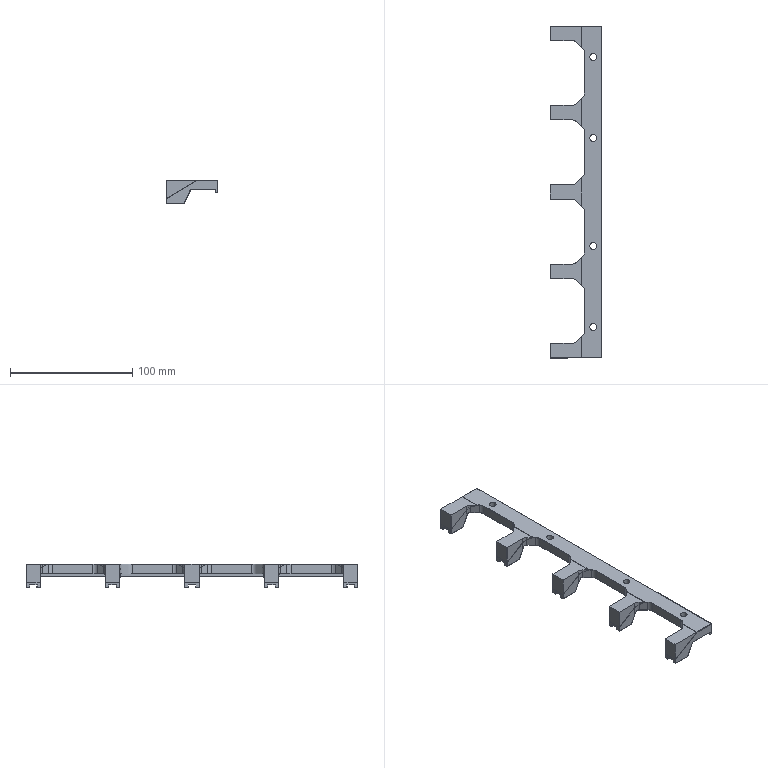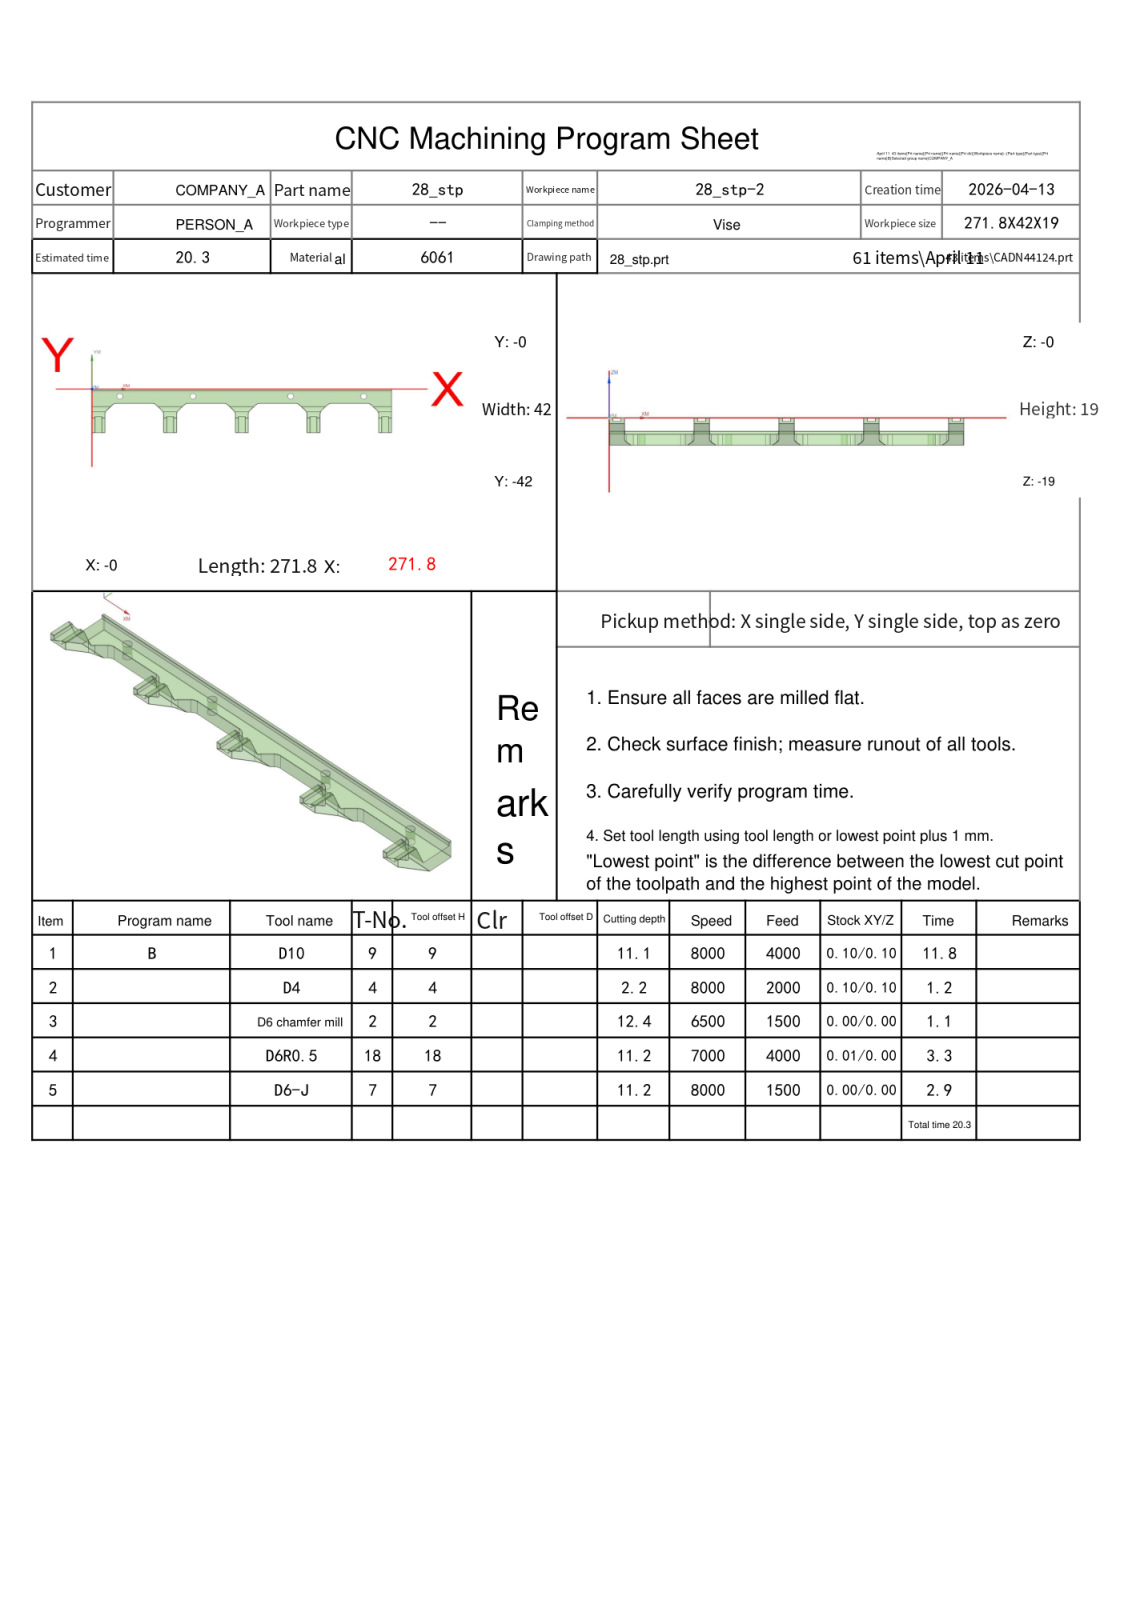NC program | NX | posted by the shop | part box 42 x 271.8 x 19 mm
Lines 1 to 789 of 14465:
%
O0001
(Machine time: 21.21 MIN)
(===Total Tool:5===)
(T9=D10     D=10.  R=0.   D-  H09 Z=-11.15)
(T4=D4      D=4.   R=0.   D-  H04 Z=-2.2  )
(T2=D6 chamfer mill   D=6.   R=0.   D-  H02 Z=-12.45)
(T18=D6R0.5 D=6.   R=0.5  D-  H18 Z=-11.25)
(T7=D6-J    D=6.   R=0.   D7  H07 Z=-11.25)
G80 G90 G17 G49 G40
G91 G28 Z0
M01
N1 T09 M06
(D10  D=10. R=0. H=09 ce=0.12 di=0.10)
G00 G90 G54 X-11.795 Y7.409 M03 S8000
G43 H09 Z20.
M08
Z2.1
G01 X-11.7 Y7.377 Z1.476 F4000.
X-11.606 Y7.345 Z1.228
X-11.511 Y7.313 Z1.046
X-11.416 Y7.281 Z.9
X-11.321 Y7.249 Z.777
X-11.227 Y7.218 Z.672
X-11.132 Y7.186 Z.58
X-11.037 Y7.154 Z.5
X-10.942 Y7.122 Z.43
X-10.847 Y7.09 Z.368
X-10.753 Y7.058 Z.314
X-10.658 Y7.026 Z.267
X-10.563 Y6.994 Z.227
X-10.468 Y6.962 Z.192
X-10.373 Y6.931 Z.164
X-10.279 Y6.899 Z.14
X-10.184 Y6.867 Z.123
X-10.089 Y6.835 Z.11
X-9.994 Y6.803 Z.103
X-9.9 Y6.771 Z.1
X-7.678 Y6.024
X-7.519 Y5.999
G03 X-7.265 Y6.065 I0.0 J.518
G02 X-4.273 Y7.054 I3.98 J-7.02
X1.978 Y7.487 I6.251 J-44.913
X2.707 Y7.481 I0.0 J-45.346
G01 X272.969 Y7.484
G02 X279.225 Y3.048 I-.106 J-6.778
X280.279 Y-2.628 I-16.186 J-5.943
X280.412 Y-11.519 I-296.3 J-8.891
X280.4 Y-14.276 I-296.434 J0.0
G01 X280.384 Y-42.069
G02 X275.948 Y-48.325 I-6.779 J.106
X270.272 Y-49.38 I-5.943 J16.179
X261.642 Y-49.511 I-8.63 J283.705
X259.174 Y-49.5 I0.0 J283.836
G01 X-1.169 Y-49.484
G02 X-7.425 Y-45.046 I.106 J6.779
X-8.479 Y-39.369 I16.195 J5.942
X-8.613 Y-30.479 I296.233 J8.891
X-8.6 Y-27.721 I296.367 J0.0
G01 X-8.579 Y.169
G02 X-5.27 Y5.129 I6.366 J-.663
X.261 Y6.734 I6.404 J-11.735
X8.124 Y7.016 I7.863 J-109.656
X10.104 Y6.998 I0.0 J-109.937
G01 X271.455 Y6.983
G02 X278.208 Y2.545 I-.199 J-7.66
X279.692 Y-3.639 I-15.009 J-6.873
X279.908 Y-11.563 I-145.435 J-7.924
X279.897 Y-13.335 I-145.651 J0.0
G01 X279.883 Y-40.554
G02 X275.445 Y-47.308 I-7.661 J.199
X269.26 Y-48.793 I-6.87 J14.988
X261.53 Y-49.006 I-7.73 J140.023
X259.965 Y-48.997 I0.0 J140.236
G01 X.346 Y-48.983
G02 X-6.409 Y-44.543 I.199 J7.66
X-7.892 Y-38.359 I14.999 J6.869
X-8.106 Y-30.635 I139.817 J7.723
X-8.097 Y-29.063 I140.03 J0.0
G01 X-8.074 Y-1.596
G02 X-3.705 Y4.686 I7.728 J-.715
X2.557 Y6.264 I7.074 J-14.863
X10.377 Y6.505 I7.82 J-126.46
X11.852 Y6.497 I0.0 J-126.702
G01 X270.151 Y6.476
G02 X277.677 Y1.337 I-.33 J-8.563
X279.179 Y-5.206 I-16.982 J-7.342
X279.406 Y-13.448 I-149.533 J-8.242
X279.396 Y-15.151 I-149.76 J0.0
G01 X279.375 Y-39.251
G02 X274.237 Y-46.777 I-8.564 J.33
X267.694 Y-48.279 I-7.34 J16.973
X259.451 Y-48.507 I-8.243 J149.431
X257.749 Y-48.497 I0.0 J149.659
G01 X1.649 Y-48.476
G02 X-5.878 Y-43.335 I.329 J8.563
X-7.379 Y-36.793 I16.987 J7.341
X-7.606 Y-28.55 I149.608 J8.243
X-7.597 Y-26.847 I149.835 J0.0
G01 X-7.583 Y-3.397
G02 X-2.472 Y4.191 I8.651 J-.311
X3.907 Y5.74 I7.394 J-16.544
X12.623 Y6.012 I8.716 J-139.521
X14.651 Y5.997 I0.0 J-139.793
G01 X268.651 Y5.98
G02 X277.155 Y.266 I-.078 J-9.301
X278.671 Y-6.584 I-18.644 J-7.719
X278.919 Y-16.462 I-196.83 J-9.878
X278.898 Y-19.329 I-197.078 J0.0
G01 X278.874 Y-37.879
G02 X273.167 Y-46.254 I-9.29 J.198
X266.317 Y-47.771 I-7.72 J18.631
X256.444 Y-48.02 I-9.873 J196.342
X253.572 Y-47.999 I0.0 J196.591
G01 X3.022 Y-47.974
G02 X-5.355 Y-42.265 I.197 J9.289
X-6.871 Y-35.416 I18.638 J7.719
X-7.119 Y-25.54 I196.76 J9.876
X-7.098 Y-22.67 I197.007 J0.0
G01 X-7.076 Y-4.721
G02 X-1.344 Y3.71 I9.379 J-.213
X5.45 Y5.252 I7.777 J-18.529
X14.088 Y5.506 I8.638 J-146.637
X15.795 Y5.496 I0.0 J-146.891
G01 X267.395 Y5.477
X267.455
G02 X276.622 Y-.684 I0.0 J-9.9
X278.154 Y-7.684 I-19.759 J-7.994
X278.414 Y-17.274 I-176.987 J-9.59
X278.397 Y-19.729 I-177.247 J0.0
X278.422 Y-26.265 I-849.199 J-6.536
X278.355 Y-36.928 I-849.224 J0.0
X272.171 Y-45.741 I-9.867 J.347
X265.217 Y-47.255 I-7.965 J19.865
X255.655 Y-47.514 I-9.562 J175.951
X253.222 Y-47.497 I0.0 J176.21
G01 X4.472 Y-47.48
X4.373
G02 X-4.901 Y-41.132 I0.0 J9.949
X-6.38 Y-33.967 I20.78 J8.025
X-6.61 Y-24.59 I191.061 J9.376
X-6.597 Y-22.321 I191.291 J0.0
X-6.623 Y-15.96 I780.546 J6.36
X-6.555 Y-5.645 I780.572 J0.0
X-.396 Y3.184 I9.936 J-.368
X6.8 Y4.757 I8.151 J-20.038
X16.203 Y5.011 I9.403 J-174.325
X18.395 Y4.997 I0.0 J-174.578
G01 X266.195 Y4.976
X266.308 Y4.977
G02 X273.054 Y2.608 I0.0 J-10.793
X276.86 Y-3.79 I-8.179 J-9.195
X277.795 Y-11.517 I-34.244 J-8.065
X277.918 Y-25.662 I-814.582 J-14.145
X277.856 Y-35.716 I-814.705 J0.0
X271.382 Y-45.169 I-10.365 J.155
X264.036 Y-46.753 I-8.341 J20.865
X254.233 Y-47.013 I-9.802 J184.172
X251.791 Y-46.997 I0.0 J184.433
G01 X5.691 Y-46.978
X5.535 Y-46.979
G02 X-.994 Y-44.818 I0.0 J10.942
X-5.025 Y-38.337 I7.733 J9.303
X-5.992 Y-30.565 I33.429 J8.107
X-6.119 Y-16.3 I800.504 J14.265
X-6.066 Y-7.066 I800.631 J0.0
X-2.953 Y.4 I10.54 J-.012
X3.803 Y3.699 I9.122 J-10.117
X12.12 Y4.443 I8.317 J-46.089
G01 X12.308
X23.358 Y4.498
X264.958 Y4.478
X265.132 Y4.479
G02 X271.26 Y2.813 I0.0 J-12.108
X276.047 Y-3.693 I-6.503 J-9.798
X277.251 Y-11.629 I-29.197 J-8.486
X277.41 Y-22.376 I-362.331 J-10.748
X277.398 Y-25.377 I-362.49 J0.0
X277.419 Y-28.555 I-231.25 J-3.178
X277.329 Y-35.025 I-231.271 J0.0
X270.515 Y-44.655 I-10.77 J.395
X263.264 Y-46.225 I-8.45 J21.495
X253.3 Y-46.513 I-9.964 J172.438
X250.92 Y-46.496 I0.0 J172.726
G01 X6.87 Y-46.478
X6.674 Y-46.48
G02 X.522 Y-44.801 I0.0 J12.114
X-4.265 Y-38.251 I6.536 J9.802
X-5.449 Y-30.413 I29.275 J8.428
X-5.612 Y-19.358 I374.413 J11.054
X-5.598 Y-16.114 I374.576 J0.0
X-5.62 Y-13.324 I170.908 J2.79
X-5.518 Y-7.416 I170.931 J0.0
X1.292 Y2.122 I10.815 J-.521
X8.787 Y3.734 I8.609 J-21.797
X18.671 Y4.011 I9.883 J-176.508
X20.932 Y3.996 I0.0 J-176.784
G01 X263.905 Y3.976
X264.088 Y3.977
G02 X270.164 Y2.482 I0.0 J-13.091
X275.365 Y-4.047 I-6.028 J-10.138
X276.713 Y-12.006 I-27.321 J-8.722
X276.917 Y-23.485 I-323.515 J-11.479
X276.897 Y-27.054 I-323.719 J0.0
X276.92 Y-29.233 I-104.221 J-2.18
X276.787 Y-34.501 I-104.244 J0.0
X269.875 Y-44.06 I-11.065 J.722
X262.191 Y-45.727 I-8.823 J22.133
X251.868 Y-46.013 I-10.323 J185.754
X249.347 Y-45.996 I0.0 J186.041
G01 X7.997 Y-45.978
G02 X7.765 Y-45.98 I-.231 J13.325
X1.768 Y-44.554 I0.0 J13.327
X-3.565 Y-37.952 I5.864 J10.192
X-4.893 Y-30.342 I26.599 J8.561
X-5.11 Y-19.961 I247.561 J10.381
X-5.097 Y-17.346 I247.779 J0.0
X-5.117 Y-14.552 I192.949 J2.793
X-5.022 Y-8.497 I192.97 J0.0
X-1.22 Y-.427 I11.218 J-.354
X5.74 Y2.7 I9.442 J-11.706
X14.298 Y3.434 I8.572 J-49.713
X23.691 Y3.501 I9.394 J-662.247
X25.697 Y3.498 I0.0 J-662.314
G01 X262.805 Y3.476
G02 X263.03 Y3.478 I.226 J-14.34
X269.016 Y2.17 I0.0 J-14.342
X274.731 Y-4.522 I-5.534 J-10.512
X276.159 Y-12.166 I-25.742 J-8.767
X276.408 Y-22.419 I-211.138 J-10.253
X276.395 Y-24.761 I-211.386 J0.0
X276.418 Y-27.455 I-156.525 J-2.694
X276.313 Y-33.209 I-156.548 J0.0
X273.046 Y-40.917 I-11.648 J.391
X266.214 Y-44.489 I-9.743 J10.319
X257.427 Y-45.412 I-8.907 J42.496
X246.757 Y-45.499 I-10.67 J655.992
X245.428 Y-45.497 I0.0 J656.079
G01 X8.978 Y-45.475
G02 X8.75 Y-45.477 I-.229 J14.212
X2.681 Y-44.117 I0.0 J14.213
X-2.918 Y-37.512 I5.642 J10.459
X-4.367 Y-29.724 I25.844 J8.838
X-4.609 Y-19.332 I222.743 J10.392
X-4.596 Y-16.878 I222.985 J0.0
X-4.618 Y-14.578 I117.791 J2.3
X-4.49 Y-9.081 I117.813 J0.0
X2.884 Y1.09 I11.518 J-.592
X10.332 Y2.695 I8.839 J-22.927
X20.903 Y3.014 I10.571 J-175.375
X23.425 Y2.995 I0.0 J-175.694
G01 X261.905 Y2.973
G02 X262.115 Y2.974 I.21 J-15.017
X268.267 Y1.656 I0.0 J-15.019
X274.158 Y-5.138 I-5.544 J-10.758
X275.637 Y-12.82 I-25.698 J-8.931
X275.906 Y-23.079 I-195.35 J-10.259
X275.894 Y-25.265 I-195.619 J0.0
X275.919 Y-27.43 I-95.331 J-2.165
X275.767 Y-32.811 I-95.356 J0.0
X268.294 Y-43.045 I-11.723 J.715
X260.353 Y-44.717 I-9.163 J23.825
X249.624 Y-45.012 I-10.729 J194.642
X247.059 Y-44.995 I0.0 J194.938
G01 X10.009 Y-44.975
G02 X9.755 Y-44.978 I-.255 J15.393
X3.726 Y-43.748 I0.0 J15.396
X-2.268 Y-37.094 I5.258 J10.763
X-3.837 Y-29.179 I25.069 J9.084
X-4.108 Y-18.729 I201.282 J10.45
X-4.095 Y-16.385 I201.553 J0.0
X-4.12 Y-14.517 I67.551 J1.868
X-3.922 Y-9.341 I67.577 J0.0
X3.602 Y.559 I11.731 J-1.107
X11.546 Y2.217 I9.178 J-24.114
X21.562 Y2.504 I10.015 J-174.607
X23.441 Y2.494 I0.0 J-174.894
G01 X260.755 Y2.477
G02 X261.039 Y2.479 I.285 J-16.818
X266.973 Y1.398 I0.0 J-16.821
X273.468 Y-5.437 I-4.84 J-11.103
X275.122 Y-13.538 I-25.006 J-9.323
X275.41 Y-24.378 I-203.341 J-10.84
X275.394 Y-26.932 I-203.629 J0.0
X275.417 Y-28.254 I-38.553 J-1.322
X275.084 Y-33.316 I-38.576 J0.0
X267.811 Y-42.421 I-11.724 J1.908
X260.138 Y-44.157 I-9.207 J22.861
X249.958 Y-44.503 I-10.18 J149.811
X248.097 Y-44.491 I0.0 J150.157
G01 X10.847 Y-44.471
G02 X10.626 Y-44.473 I-.221 J15.999
X4.462 Y-43.238 I0.0 J16.
X-1.762 Y-36.33 I5.305 J11.037
X-3.325 Y-28.411 I25.671 J9.182
X-3.61 Y-17.523 I207.847 J10.888
X-3.518 Y-11.318 I208.132 J0.0
X-1.305 Y-4.308 I13.227 J-.322
X5.76 Y.56 I10.658 J-7.907
X14.093 Y1.82 I9.163 J-32.428
X24.897 Y2.006 I10.804 J-312.688
X27.39 Y1.996 I0.0 J-312.874
G01 X259.655 Y1.979
G02 X260.007 Y1.983 I.352 J-18.624
X265.853 Y1.041 I0.0 J-18.627
X272.898 Y-6.019 I-4.401 J-11.437
X274.593 Y-14.06 I-24.769 J-9.42
X274.906 Y-24.501 I-173.985 J-10.441
X274.797 Y-30.652 I-174.298 J0.0
X272.374 Y-37.853 I-13.237 J.446
X265.423 Y-42.529 I-10.66 J8.341
X256.843 Y-43.821 I-9.368 J33.069
X244.891 Y-44.013 I-11.951 J372.933
X241.395 Y-43.996 I0.0 J373.125
G01 X11.845 Y-43.972
G02 X11.581 Y-43.974 I-.264 J17.171
X5.389 Y-42.819 I0.0 J17.173
X-1.193 Y-35.748 I5.067 J11.315
X-2.793 Y-27.939 I25.367 J9.266
X-3.099 Y-17.692 I171.118 J10.247
X-3.006 Y-12.047 I171.425 J0.0
X-.751 Y-4.932 I13.547 J-.379
X6.244 Y-.032 I10.784 J-7.953
X14.415 Y1.287 I9.237 J-31.246
X25.947 Y1.513 I11.532 J-294.663
X29.112 Y1.496 I0.0 J-294.889
G01 X258.862 Y1.476
G02 X259.212 Y1.479 I.351 J-18.864
X265.347 Y.454 I0.0 J-18.867
X272.345 Y-6.626 I-4.624 J-11.569
X274.075 Y-14.709 I-24.857 J-9.547
X274.394 Y-24.373 I-146.526 J-9.663
X274.292 Y-29.85 I-146.844 J0.0
X271.94 Y-37.079 I-13.678 J.453
X264.819 Y-41.98 I-10.907 J8.221
X256.295 Y-43.303 I-9.448 J32.751
X244.601 Y-43.511 I-11.694 J328.735
X241.398 Y-43.496 I0.0 J328.943
G01 X13.148 Y-43.48
G02 X12.741 Y-43.484 I-.407 J20.026
X6.838 Y-42.594 I0.0 J20.03
X-.545 Y-35.373 I4.21 J11.69
X-2.275 Y-27.29 I24.856 J9.546
X-2.59 Y-17.957 I138.294 J9.332
X-2.49 Y-12.699 I138.609 J0.0
X-.148 Y-5.47 I13.742 J-.46
X6.955 Y-.545 I10.936 J-8.186
X15.577 Y.803 I9.529 J-32.693
X27.763 Y1.015 I12.186 J-351.327
X31.374 Y.996 I0.0 J-351.538
G01 X258.124 Y.972
G02 X258.427 Y.975 I.303 J-19.32
X264.66 Y-.058 I0.0 J-19.323
X271.866 Y-7.394 I-4.675 J-11.8
X273.579 Y-15.589 I-25.787 J-9.668
X273.887 Y-23.974 I-114.061 J-8.386
X273.757 Y-29.429 I-114.368 J0.0
X271.04 Y-36.938 I-13.49 J.634
X263.709 Y-41.594 I-10.961 J9.159
X255.116 Y-42.819 I-9.484 J35.776
X243.422 Y-43.009 I-11.693 J360.837
X240.318 Y-42.995 I0.0 J361.026
G01 X13.818 Y-42.975
G02 X13.484 Y-42.978 I-.334 J20.139
X7.414 Y-42.042 I0.0 J20.142
X.011 Y-34.79 I4.341 J11.837
X-1.736 Y-26.908 I24.518 J9.568
X-2.077 Y-18.213 I110.618 J8.696
X-1.967 Y-13.269 I110.96 J0.0
X.6 Y-5.803 I13.757 J-.556
X7.78 Y-1.016 I11.006 J-8.728
X16.608 Y.312 I9.687 J-34.392
X28.879 Y.513 I12.271 J-374.296
X32.506 Y.496 I0.0 J-374.497
G01 X257.105 Y.475
G02 X257.479 Y.478 I.374 J-20.932
X263.709 Y-.47 I0.0 J-20.935
X271.264 Y-7.851 I-4.361 J-12.02
X273.025 Y-15.777 I-24.796 J-9.67
X273.368 Y-23.848 I-94.987 J-8.071
X273.241 Y-28.765 I-95.329 J0.0
X270.383 Y-36.48 I-13.646 J.668
X263.117 Y-41.054 I-11.013 J9.437
X254.429 Y-42.312 I-9.626 J35.863
X242.438 Y-42.51 I-11.991 J361.696
X239.131 Y-42.495 I0.0 J361.895
G01 X14.582 Y-42.472
G02 X14.25 Y-42.475 I-.331 J20.452
X7.984 Y-41.492 I0.0 J20.455
X.536 Y-34.148 I4.474 J11.987
X-1.225 Y-26.221 I24.804 J9.67
X-1.56 Y-18.463 I89.769 J7.758
X-1.438 Y-13.783 I90.104 J0.0
X1.31 Y-6.185 I13.752 J-.679
X8.625 Y-1.478 I11.102 J-9.213
X17.26 Y-.197 I9.636 J-35.228
X29.588 Y.013 I12.328 J-361.145
X33.157 Y-.005 I0.0 J-361.355
G01 X256.257 Y-.025
G02 X256.641 Y-.022 I.384 J-21.962
X262.918 Y-.938 I0.0 J-21.965
X270.752 Y-8.512 I-4.26 J-12.246
X272.545 Y-16.786 I-25.686 J-9.896
X272.843 Y-23.698 I-79.8 J-6.912
X272.721 Y-28.125 I-80.098 J0.0
X269.844 Y-35.884 I-13.824 J.714
X262.41 Y-40.552 I-11.184 J9.555
X253.519 Y-41.816 I-9.785 J36.946
X240.923 Y-42.012 I-12.597 J403.156
X237.172 Y-41.995 I0.0 J403.353
G01 X15.572 Y-41.975
G02 X15.178 Y-41.978 I-.394 J22.095
X8.91 Y-41.071 I0.0 J22.099
X1.048 Y-33.487 I4.231 J12.254
X-.722 Y-25.462 I25.29 J9.787
X-1.038 Y-18.742 I71.335 J6.719
X-.889 Y-14.125 I71.651 J0.0
X2.437 Y-6.088 I13.46 J-.864
X9.987 Y-1.793 I11.065 J-10.666
X19.15 Y-.649 I9.828 J-41.452
X30.542 Y-.499 I11.392 J-434.014
X32.848 Y-.505 I0.0 J-434.163
G01 X255.098 Y-.52
G02 X255.595 Y-.515 I.497 J-24.834
X261.781 Y-1.298 I0.0 J-24.839
X270.19 Y-9.041 I-3.761 J-12.521
X272.031 Y-17.405 I-25.68 J-10.038
X272.318 Y-23.433 I-63.226 J-6.028
X272.164 Y-27.843 I-63.513 J0.0
X268.641 Y-36.051 I-13.485 J.929
X261.267 Y-40.176 I-11.01 J11.026
X252.109 Y-41.343 I-9.893 J41.149
X239.832 Y-41.506 I-12.277 J460.42
X236.561 Y-41.495 I0.0 J460.583
G01 X16.211 Y-41.471
G02 X15.887 Y-41.473 I-.324 J22.324
X9.551 Y-40.555 I0.0 J22.327
X1.61 Y-32.958 I4.246 J12.386
X-.231 Y-24.594 I25.683 J10.038
X-.509 Y-18.952 I57.129 J5.641
X-.333 Y-14.458 I57.407 J0.0
X3.94 Y-5.721 I13.217 J-1.051
X11.597 Y-2.072 I10.862 J-12.934
X20.784 Y-1.119 I9.751 J-49.243
X32.79 Y-1.001 I12.006 J-611.267
X35.033 Y-1.005 I0.0 J-611.385
G01 X254.833 Y-1.031
G02 X255.161 Y-1.028 I.328 J-22.802
X261.642 Y-1.968 I0.0 J-22.804
X269.612 Y-9.526 I-4.277 J-12.493
X271.5 Y-17.828 I-25.254 J-10.11
X271.784 Y-23.209 I-50.985 J-5.38
X271.598 Y-27.563 I-51.268 J0.0
X266.537 Y-36.874 I-13.169 J1.127
X258.835 Y-40.076 I-10.698 J14.867
X248.833 Y-40.919 I-10.085 J59.858
X238.679 Y-40.996 I-10.153 J670.923
X236.933 Y-40.994 I0.0 J671.
G01 X17.083 Y-40.971
G02 X16.705 Y-40.974 I-.378 J23.254
X10.221 Y-40.052 I0.0 J23.257
X2.188 Y-32.473 I4.216 J12.516
X.304 Y-24.221 I25.172 J10.087
X.029 Y-19.158 I46.457 J5.063
X.239 Y-14.737 I46.732 J0.0
X8.483 Y-3.781 I13.175 J-1.333
X16.84 Y-1.893 I10.143 J-25.469
X27.614 Y-1.506 I10.775 J-149.721
X29.13 Y-1.514 I0.0 J-150.108
G01 X253.98 Y-1.53
G02 X254.344 Y-1.527 I.364 J-23.886
X260.894 Y-2.442 I0.0 J-23.889
X269.12 Y-10.201 I-4.194 J-12.686
X270.981 Y-18.365 I-25.435 J-10.092
X271.24 Y-23.021 I-41.625 J-4.656
X271.021 Y-27.298 I-41.884 J0.0
X262.748 Y-38.196 I-13.235 J1.458
X254.394 Y-40.095 I-10.196 J25.53
X243.374 Y-40.495 I-11.02 J151.412
X241.654 Y-40.485 I0.0 J151.812
G01 X18.204 Y-40.477
G02 X17.719 Y-40.481 I-.485 J26.141
X11.369 Y-39.698 I0.0 J26.145
X2.68 Y-31.798 I3.722 J12.821
X.789 Y-23.292 I25.918 J10.227
X.574 Y-19.32 I36.568 J3.972
X.851 Y-14.811 I36.784 J0.0
X9.025 Y-4.33 I13.164 J-1.839
X17.175 Y-2.432 I10.131 J-25.049
X28.289 Y-2.005 I11.114 J-144.273
X29.964 Y-2.014 I0.0 J-144.701
G01 X253.214 Y-2.03
G02 X253.584 Y-2.027 I.371 J-24.668
X260.181 Y-2.926 I0.0 J-24.671
X268.556 Y-10.702 I-4.109 J-12.823
X270.496 Y-19.298 I-25.697 J-10.316
X270.692 Y-22.857 I-32.272 J-3.559
X270.369 Y-27.425 I-32.468 J0.0
X262.164 Y-37.667 I-13.183 J2.154
X253.56 Y-39.604 I-10.372 J25.987
X242.602 Y-39.992 I-10.958 J154.469
X241.019 Y-39.984 I0.0 J154.857
G01 X18.619 Y-39.97
G02 X18.241 Y-39.973 I-.379 J24.856
X11.65 Y-39.083 I0.0 J24.859
X3.244 Y-31.297 I4.078 J12.833
X1.316 Y-22.801 I25.463 J10.246
X1.13 Y-19.477 I29.725 J3.324
X1.494 Y-14.827 I29.911 J0.0
X9.431 Y-4.938 I13.09 J-2.376
X17.862 Y-2.936 I10.358 J-24.863
X29.274 Y-2.501 I11.412 J-149.662
X31.201 Y-2.514 I0.0 J-150.097
G01 X252.451 Y-2.531
G02 X252.796 Y-2.528 I.345 J-25.909
X259.329 Y-3.366 I0.0 J-25.912
X268.079 Y-11.395 I-3.91 J-13.043
X270.022 Y-20.499 I-26.463 J-10.407
X270.135 Y-22.829 I-23.977 J-2.33
X269.551 Y-28.102 I-24.09 J0.0
X261.705 Y-37.085 I-12.939 J3.383
X253.468 Y-39.044 I-10.297 J25.003
X241.998 Y-39.496 I-11.47 J145.119
X240.13 Y-39.484 I0.0 J145.571
G01 X19.431 Y-39.47
G02 X19.055 Y-39.473 I-.375 J26.33
X12.549 Y-38.657 I0.0 J26.333
X3.721 Y-30.604 I3.832 J13.066
X1.788 Y-21.499 I26.123 J10.305
X1.691 Y-19.449 I21.654 J2.05
X2.433 Y-13.817 I21.751 J0.0
X10.162 Y-5.398 I12.802 J-3.996
X18.652 Y-3.428 I10.408 J-25.577
X29.787 Y-3.008 I11.134 J-147.205
X31.392 Y-3.016 I0.0 J-147.625
G01 X251.341 Y-3.025
G02 X251.84 Y-3.021 I.498 J-28.443
X258.43 Y-3.794 I0.0 J-28.447
X267.508 Y-11.864 I-3.62 J-13.213
X269.497 Y-21.359 I-25.617 J-10.323
X269.557 Y-22.861 I-18.894 J-1.502
X268.537 Y-28.994 I-18.954 J0.0
X261.024 Y-36.604 I-12.606 J4.932
X252.426 Y-38.577 I-10.488 J25.989
X240.877 Y-38.997 I-11.549 J158.47
X238.937 Y-38.985 I0.0 J158.89
G01 X20.387 Y-38.973
G02 X19.909 Y-38.977 I-.477 J27.972
X13.301 Y-38.186 I0.0 J27.976
X4.292 Y-30.135 I3.688 J13.193
X2.309 Y-19.948 I25.176 J10.187
X2.583 Y-16.102 I27.159 J0.0
X10.569 Y-6.001 I13.201 J-2.229
X18.991 Y-3.965 I10.474 J-24.883
X29.836 Y-3.518 I10.845 J-131.274
X30.979 Y-3.523 I0.0 J-131.722
G01 X250.778 Y-3.528
G02 X251.222 Y-3.525 I.444 J-28.201
X257.914 Y-4.33 I0.0 J-28.204
X267.054 Y-12.599 I-3.754 J-13.337
X268.926 Y-22.241 I-23.907 J-9.643
X268.679 Y-25.799 I-25.778 J0.0
X260.839 Y-35.901 I-13.194 J2.146
X252.284 Y-38.021 I-10.608 J24.486
X241.176 Y-38.485 I-11.109 J132.924
X239.848 Y-38.478 I0.0 J133.387
G01 X21.148 Y-38.473
G02 X20.66 Y-38.477 I-.488 J28.958
X14.008 Y-37.703 I0.0 J28.962
X4.746 Y-29.4 I3.631 J13.368
X2.918 Y-20.116 I22.658 J9.284
X3.186 Y-16.498 I24.486 J0.0
X11.116 Y-6.541 I13.168 J-2.35
X19.585 Y-4.475 I10.551 J-24.866
X30.654 Y-4.016 I11.069 J-133.105
X31.922 Y-4.022 I0.0 J-133.564
G01 X249.821 Y-4.025
G02 X250.341 Y-4.021 I.519 J-30.5
X257.016 Y-4.76 I0.0 J-30.504
X266.545 Y-13.199 I-3.475 J-13.523
X268.308 Y-22.071 I-21.436 J-8.872
X268.06 Y-25.456 I-23.2 J0.0
X260.338 Y-35.341 I-13.13 J2.299
X251.842 Y-37.495 I-10.645 J24.155
X240.846 Y-37.978 I-10.997 J124.902
X239.757 Y-37.974 I0.0 J125.385
G01 X21.907 Y-37.973
G02 X21.418 Y-37.977 I-.489 J30.166
X14.763 Y-37.234 I0.0 J30.17
X5.255 Y-28.798 I3.493 J13.512
X3.544 Y-20.263 I20.43 J8.535
X3.796 Y-16.935 I22.142 J0.0
X11.53 Y-7.14 I13.088 J-2.384
X20.074 Y-4.996 I10.665 J-24.398
X31.321 Y-4.515 I11.246 J-131.404
X32.66 Y-4.522 I0.0 J-131.884
G01 X249.16 Y-4.526
G02 X249.651 Y-4.522 I.491 J-31.109
X256.357 Y-5.253 I0.0 J-31.113
X266.045 Y-13.82 I-3.428 J-13.639
X267.673 Y-21.885 I-19.168 J-8.065
X267.392 Y-25.29 I-20.795 J0.0
X259.923 Y-34.74 I-12.981 J2.584
X251.498 Y-36.958 I-10.697 J23.52
X239.969 Y-37.484 I-11.529 J125.997
X238.514 Y-37.476 I0.0 J126.524
G01 X22.315 Y-37.467
G02 X21.908 Y-37.47 I-.407 J28.784
X15.081 Y-36.649 I0.0 J28.787
X5.814 Y-28.315 I3.761 J13.502
X4.188 Y-20.457 I18.179 J7.858
X4.492 Y-17.001 I19.804 J0.0
X11.937 Y-7.745 I12.913 J-2.765
X20.366 Y-5.539 I10.693 J-23.644
X31.406 Y-5.025 I11.04 J-118.368
X32.35 Y-5.029 I0.0 J-118.881
G01 X248.6
G02 X249.084 Y-5.025 I.484 J-30.351
X255.988 Y-5.821 I0.0 J-30.355
X265.506 Y-14.349 I-3.638 J-13.635
X267.017 Y-21.707 I-17.155 J-7.359
X266.692 Y-25.176 I-18.667 J0.0
X259.434 Y-34.173 I-12.814 J2.912
X250.923 Y-36.447 I-10.783 J23.295
X239.517 Y-36.98 I-11.406 J121.821
X238.24 Y-36.973 I0.0 J122.354
G01 X23.29 Y-36.972
G02 X22.81 Y-36.975 I-.48 J31.474
X16.044 Y-36.239 I0.0 J31.477
X6.275 Y-27.594 I3.41 J13.695
X4.853 Y-20.624 I16.368 J6.969
X5.194 Y-17.157 I17.79 J0.0
X12.441 Y-8.306 I12.735 J-3.034
X20.864 Y-6.059 I10.738 J-23.341
X32.137 Y-5.523 I11.274 J-118.426
X33.196 Y-5.528 I0.0 J-118.961
G01 X248.096 Y-5.533
G02 X248.482 Y-5.53 I.386 J-30.421
X255.337 Y-6.312 I0.0 J-30.424
X265.078 Y-15.164 I-3.591 J-13.739
X266.342 Y-21.534 I-15.43 J-6.371
X265.941 Y-25.169 I-16.694 J0.0
X258.788 Y-33.683 I-12.632 J3.351
X250.275 Y-35.945 I-10.794 J23.473
X239.181 Y-36.471 I-11.095 J116.747
X238.292 Y-36.467 I0.0 J117.273
G01 X23.843 Y-36.469
G02 X23.379 Y-36.472 I-.463 J30.819
X16.453 Y-35.684 I0.0 J30.822
X6.643 Y-26.607 I3.611 J13.742
X5.538 Y-20.806 I14.675 J5.801
X6.021 Y-16.932 I15.779 J0.0
X12.878 Y-8.901 I12.447 J-3.686
X21.281 Y-6.588 I10.786 J-22.761
X32.618 Y-6.026 I11.337 J-113.97
X33.662 Y-6.031 I0.0 J-114.533
G01 X247.162 Y-6.029
G02 X247.647 Y-6.025 I.485 J-32.43
X254.558 Y-6.77 I0.0 J-32.434
X264.653 Y-16.029 I-3.383 J-13.821
X265.645 Y-21.354 I-13.79 J-5.324
X265.008 Y-25.646 I-14.783 J0.0
X258.124 Y-33.2 I-12.323 J4.316
X249.798 Y-35.423 I-10.719 J23.442
X238.263 Y-35.977 I-11.535 J119.726
X237.017 Y-35.971 I0.0 J120.281
G01 X24.467 Y-35.967
G02 X24.008 Y-35.971 I-.458 J30.903
X16.98 Y-35.161 I0.0 J30.906
X6.964 Y-25.368 I3.661 J13.762
X6.24 Y-20.976 I12.953 J4.391
X7.322 Y-15.643 I13.677 J0.0
X14.285 Y-9.031 I12.097 J-5.768
X22.61 Y-7.012 I10.587 J-25.467
X33.638 Y-6.528 I11.028 J-125.404
X34.445 Y-6.53 I0.0 J-125.888
G01 X246.245 Y-6.526
G02 X246.832 Y-6.521 I.587 J-34.322
X253.845 Y-7.245 I0.0 J-34.327
X264.52 Y-18.053 I-3.258 J-13.895
X264.938 Y-21.259 I-12.076 J-3.206
X262.359 Y-28.863 I-12.494 J0.0
X254.956 Y-33.718 I-11.66 J9.706
X245.752 Y-35.222 I-10.623 J36.111
X233.439 Y-35.5 I-12.313 J272.108
X230.907 Y-35.488 I0.0 J272.387
G01 X25.457 Y-35.471
G02 X24.912 Y-35.476 I-.544 J33.892
X17.957 Y-34.755 I0.0 J33.896
X7.014 Y-21.012 I3.156 J13.742
X7.252 Y-18.433 I14.1 J0.0
X13.6 Y-10.194 I12.103 J-2.76
X21.885 Y-7.681 I10.858 J-20.886
X32.939 Y-7.046 I11.054 J-95.893
X33.411 Y-7.047 I0.0 J-96.528
G01 X44.911 Y-7.009
X245.56 Y-7.027
G02 X246.123 Y-7.022 I.562 J-35.676
X253.065 Y-7.704 I0.0 J-35.68
X264.136 Y-21.277 I-2.786 J-13.573
X264.055 Y-22.772 I-13.856 J0.0
X257.998 Y-31.577 I-11.98 J1.755
X249.766 Y-34.251 I-10.931 J19.641
X238.824 Y-34.941 I-10.942 J86.522
G01 X238.595 Y-34.94
X227.145 Y-34.99
X26.145 Y-34.971
G02 X25.567 Y-34.976 I-.578 J34.215
X18.497 Y-34.238 I0.0 J34.22
X7.775 Y-20.905 I2.929 J13.333
X7.778 Y-20.644 I13.651 J0.0
X13.455 Y-11.169 I11.778 J-.618
X21.428 Y-8.351 I10.892 J-18.131
X32.406 Y-7.571 I10.978 J-76.87
G01 X32.49
X43.74 Y-7.51
X244.84 Y-7.526
G02 X245.45 Y-7.521 I.61 J-36.246
X252.494 Y-8.212 I0.0 J-36.252
X263.16 Y-18.878 I-2.729 J-13.394
X263.352 Y-20.965 I-11.249 J-2.087
X258.246 Y-30.492 I-11.441 J0.0
X250.51 Y-33.514 I-10.91 J16.513
X239.759 Y-34.406 I-10.917 J66.377
X228.198 Y-34.496 I-11.561 J738.129
X225.16 Y-34.49 I0.0 J738.22
G01 X26.86 Y-34.471
G02 X26.301 Y-34.476 I-.558 J35.853
X19.306 Y-33.787 I0.0 J35.857
X9.288 Y-25.257 I2.713 J13.334
X8.593 Y-21.369 I10.53 J3.888
X13.472 Y-12.11 I11.225 J0.0
X21.274 Y-8.997 I10.939 J-16.079
X31.975 Y-8.096 I10.905 J-65.52
X43.363 Y-8.005 I11.388 J-715.518
X45.924 Y-8.01 I0.0 J-715.608
G01 X244.474 Y-8.031
G02 X244.955 Y-8.028 I.481 J-35.356
X251.977 Y-8.732 I0.0 J-35.359
X261.384 Y-15.963 I-2.748 J-13.309
X262.511 Y-20.809 I-9.851 J-4.847
X257.867 Y-29.777 I-10.978 J0.0
X250.383 Y-32.908 I-10.824 J15.36
X240.191 Y-33.877 I-10.717 J58.68
X227.333 Y-33.993 I-12.858 J711.528
X225.192 Y-33.99 I0.0 J711.644
G01 X27.542 Y-33.971
G02 X26.961 Y-33.976 I-.581 J36.431
X19.888 Y-33.283 I0.0 J36.436
X10.904 Y-26.889 I2.678 J13.272
X9.454 Y-21.503 I9.279 J5.385
X13.813 Y-12.871 I10.728 J0.0
X21.343 Y-9.617 I10.85 J-14.772
X31.532 Y-8.626 I10.727 J-57.39
X44.515 Y-8.506 I12.984 J-702.826
X46.881 Y-8.51 I0.0 J-702.946
G01 X243.73 Y-8.53
G02 X244.294 Y-8.526 I.564 J-35.73
X251.48 Y-9.256 I0.0 J-35.735
X259.958 Y-15.029 I-2.777 J-13.189
X261.631 Y-20.695 I-8.76 J-5.666
X257.657 Y-28.888 I-10.433 J0.0
X250.271 Y-32.286 I-10.816 J13.785
X240.393 Y-33.348 I-10.622 J52.341
X227.26 Y-33.498 I-13.133 J576.076
X224.144 Y-33.489 I0.0 J576.226
G01 X28.194 Y-33.471
G02 X27.628 Y-33.475 I-.566 J37.314
X20.538 Y-32.795 I0.0 J37.318
X12.244 Y-27.514 I2.599 J13.235
X10.356 Y-21.609 I8.287 J5.904
X14.09 Y-13.732 I10.175 J0.0
X21.298 Y-10.281 I10.728 J-13.154
X30.769 Y-9.177 I10.451 J-48.471
X44.017 Y-8.998 I13.248 J-489.976
X47.517 Y-9.01 I0.0 J-490.155
G01 X243.017 Y-9.03
G02 X243.61 Y-9.025 I.593 J-36.625
X250.868 Y-9.751 I0.0 J-36.63
X258.74 Y-14.678 I-2.702 J-13.07
X260.708 Y-20.592 I-7.903 J-5.913
X257.393 Y-27.97 I-9.87 J0.0
X250.278 Y-31.618 I-10.708 J12.122
X240.719 Y-32.808 I-10.536 J45.639
X227.191 Y-33.003 I-13.528 J469.608
X223.521 Y-32.989 I0.0 J469.803
G01 X28.771 Y-32.969